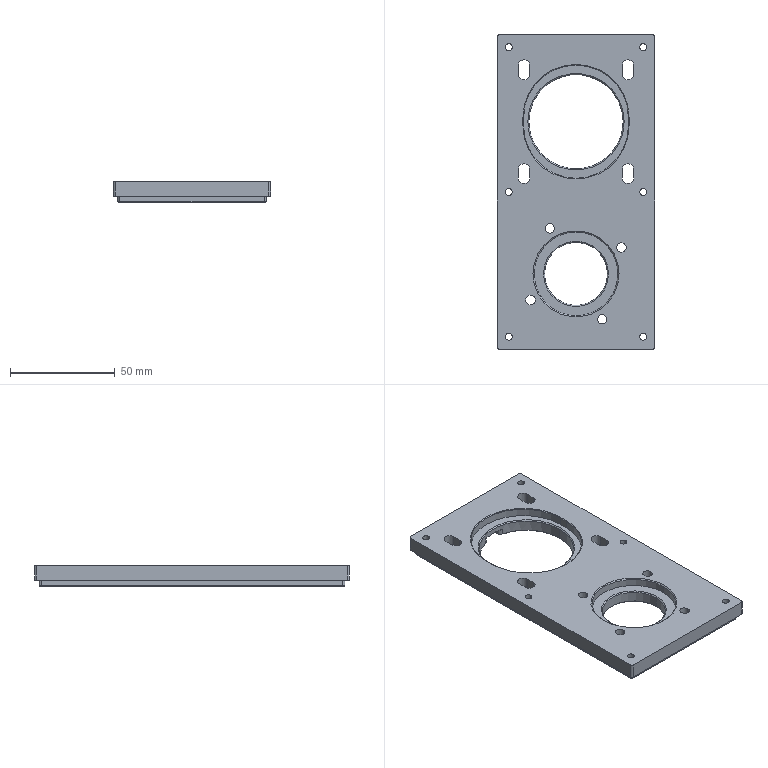Part | STEP file | 10电机Plate EDA50-R-010-D60NH-BZ^EDA50-R04 (D60N) | 1 solid | 136 faces | box 75 x 150 x 10 mm | volume 76605 mm3 | cylinder 64 | plane 51 | cone 21 | commonest cylinder face diameters 3.3 x12 2 x8 4.5 x8 5.5 x8 7.5 x8 8 x8